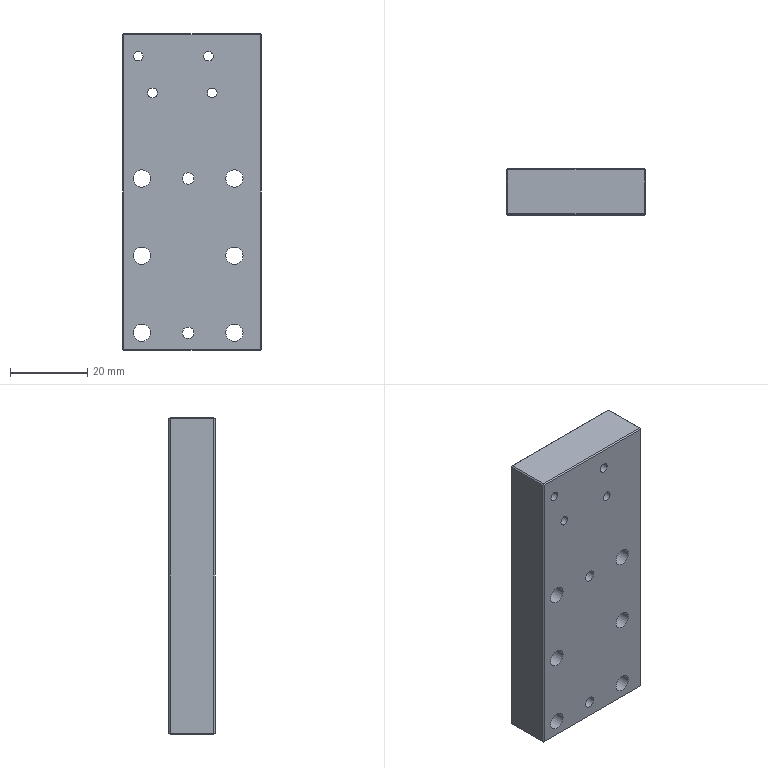Part | 1 solid | 72 faces | box 36 x 12 x 82 mm | volume 32920 mm3 | cylinder 36 | plane 24 | cone 12 | commonest cylinder face diameters 4.5 x12 8 x12 2.5 x8 3 x4